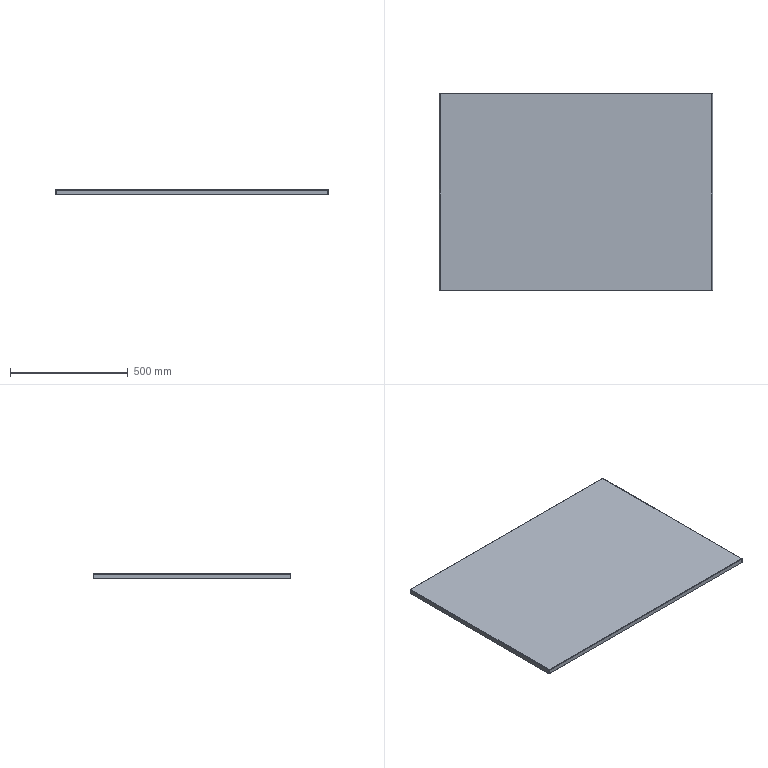Part | STEP file | Part 15 | 1 solid | 38 faces | box 1160 x 840 x 20 mm | volume 2086843 mm3 | plane 22 | spline 8 | cylinder 8 | commonest cylinder face diameters 1 x4 5 x4
STEP:
#1=CARTESIAN_POINT('',(-577.5,-417.5,-2.));
#2=VERTEX_POINT('',#1);
#3=CARTESIAN_POINT('',(577.5,-417.5,-2.));
#4=VERTEX_POINT('',#3);
#5=CARTESIAN_POINT('',(-577.5,-417.5,-2.));
#6=DIRECTION('',(1.,0.,0.));
#7=VECTOR('',#6,1000.);
#8=LINE('',#5,#7);
#9=EDGE_CURVE('',#2,#4,#8,.T.);
#10=ORIENTED_EDGE('',*,*,#9,.F.);
#11=CARTESIAN_POINT('',(-577.5,417.5,-2.));
#12=VERTEX_POINT('',#11);
#13=CARTESIAN_POINT('',(-577.5,417.5,-2.));
#14=DIRECTION('',(0.,-1.,0.));
#15=VECTOR('',#14,1000.);
#16=LINE('',#13,#15);
#17=EDGE_CURVE('',#12,#2,#16,.T.);
#18=ORIENTED_EDGE('',*,*,#17,.F.);
#19=CARTESIAN_POINT('',(577.5,417.5,-2.));
#20=VERTEX_POINT('',#19);
#21=CARTESIAN_POINT('',(577.5,417.5,-2.));
#22=DIRECTION('',(-1.,0.,0.));
#23=VECTOR('',#22,1000.);
#24=LINE('',#21,#23);
#25=EDGE_CURVE('',#20,#12,#24,.T.);
#26=ORIENTED_EDGE('',*,*,#25,.F.);
#27=CARTESIAN_POINT('',(577.5,-417.5,-2.));
#28=DIRECTION('',(0.,1.,0.));
#29=VECTOR('',#28,1000.);
#30=LINE('',#27,#29);
#31=EDGE_CURVE('',#4,#20,#30,.T.);
#32=ORIENTED_EDGE('',*,*,#31,.F.);
#33=EDGE_LOOP('',(#10,#18,#26,#32));
#34=FACE_OUTER_BOUND('',#33,.T.);
#35=CARTESIAN_POINT('',(0.,0.,-2.));
#36=DIRECTION('',(0.,0.,1.));
#37=DIRECTION('',(1.,0.,0.));
#38=AXIS2_PLACEMENT_3D('',#35,#36,#37);
#39=PLANE('',#38);
#40=ADVANCED_FACE('',(#34),#39,.F.);
#41=CARTESIAN_POINT('',(-577.5,417.5,0.));
#42=VERTEX_POINT('',#41);
#43=CARTESIAN_POINT('',(-577.5,-417.5,0.));
#44=VERTEX_POINT('',#43);
#45=CARTESIAN_POINT('',(-577.5,417.5,0.));
#46=DIRECTION('',(0.,-1.,0.));
#47=VECTOR('',#46,1000.);
#48=LINE('',#45,#47);
#49=EDGE_CURVE('',#42,#44,#48,.T.);
#50=ORIENTED_EDGE('',*,*,#49,.T.);
#51=CARTESIAN_POINT('',(577.5,-417.5,0.));
#52=VERTEX_POINT('',#51);
#53=CARTESIAN_POINT('',(-577.5,-417.5,0.));
#54=DIRECTION('',(1.,0.,0.));
#55=VECTOR('',#54,1000.);
#56=LINE('',#53,#55);
#57=EDGE_CURVE('',#44,#52,#56,.T.);
#58=ORIENTED_EDGE('',*,*,#57,.T.);
#59=CARTESIAN_POINT('',(577.5,417.5,0.));
#60=VERTEX_POINT('',#59);
#61=CARTESIAN_POINT('',(577.5,-417.5,0.));
#62=DIRECTION('',(0.,1.,0.));
#63=VECTOR('',#62,1000.);
#64=LINE('',#61,#63);
#65=EDGE_CURVE('',#52,#60,#64,.T.);
#66=ORIENTED_EDGE('',*,*,#65,.T.);
#67=CARTESIAN_POINT('',(577.5,417.5,0.));
#68=DIRECTION('',(-1.,0.,0.));
#69=VECTOR('',#68,1000.);
#70=LINE('',#67,#69);
#71=EDGE_CURVE('',#60,#42,#70,.T.);
#72=ORIENTED_EDGE('',*,*,#71,.T.);
#73=EDGE_LOOP('',(#50,#58,#66,#72));
#74=FACE_OUTER_BOUND('',#73,.T.);
#75=CARTESIAN_POINT('',(0.,0.,0.));
#76=DIRECTION('',(0.,0.,1.));
#77=DIRECTION('',(1.,0.,0.));
#78=AXIS2_PLACEMENT_3D('',#75,#76,#77);
#79=PLANE('',#78);
#80=ADVANCED_FACE('',(#74),#79,.T.);
#81=CARTESIAN_POINT('',(-577.293,420.,-2.5));
#82=VERTEX_POINT('',#81);
#83=CARTESIAN_POINT('',(-577.293,418.,-2.5));
#84=VERTEX_POINT('',#83);
#85=CARTESIAN_POINT('',(-577.293,418.,-2.5));
#86=DIRECTION('',(0.,-1.,0.));
#87=VECTOR('',#86,1000.);
#88=LINE('',#85,#87);
#89=EDGE_CURVE('',#82,#84,#88,.T.);
#90=ORIENTED_EDGE('',*,*,#89,.T.);
#91=CARTESIAN_POINT('',(-577.5,417.5,-2.));
#92=CARTESIAN_POINT('',(-577.465,417.631,-2.));
#93=CARTESIAN_POINT('',(-577.431,417.761,-2.054));
#94=CARTESIAN_POINT('',(-577.362,417.946,-2.239));
#95=CARTESIAN_POINT('',(-577.327,418.,-2.369));
#96=CARTESIAN_POINT('',(-577.293,418.,-2.5));
#97=B_SPLINE_CURVE_WITH_KNOTS('',3,(#91,#92,#93,#94,#95,#96),.UNSPECIFIED.,.F.,.F.,(4,2,4),(0.,0.5,1.),.UNSPECIFIED.);
#98=EDGE_CURVE('',#12,#84,#97,.T.);
#99=ORIENTED_EDGE('',*,*,#98,.F.);
#100=CARTESIAN_POINT('',(-577.5,417.5,-2.));
#101=DIRECTION('',(0.,0.,1.));
#102=VECTOR('',#101,1000.);
#103=LINE('',#100,#102);
#104=EDGE_CURVE('',#12,#42,#103,.T.);
#105=ORIENTED_EDGE('',*,*,#104,.T.);
#106=CARTESIAN_POINT('',(-577.5,417.5,0.));
#107=CARTESIAN_POINT('',(-577.483,417.827,0.));
#108=CARTESIAN_POINT('',(-577.465,418.154,-0.06507));
#109=CARTESIAN_POINT('',(-577.431,418.759,-0.3155));
#110=CARTESIAN_POINT('',(-577.414,419.036,-0.5008));
#111=CARTESIAN_POINT('',(-577.379,419.499,-0.9636));
#112=CARTESIAN_POINT('',(-577.362,419.684,-1.241));
#113=CARTESIAN_POINT('',(-577.327,419.935,-1.846));
#114=CARTESIAN_POINT('',(-577.31,420.,-2.173));
#115=CARTESIAN_POINT('',(-577.293,420.,-2.5));
#116=B_SPLINE_CURVE_WITH_KNOTS('',3,(#106,#107,#108,#109,#110,#111,#112,#113,#114,#115),.UNSPECIFIED.,.F.,.F.,(4,2,2,2,4),(0.,0.25,0.5,0.75,1.),.UNSPECIFIED.);
#117=EDGE_CURVE('',#42,#82,#116,.T.);
#118=ORIENTED_EDGE('',*,*,#117,.T.);
#119=EDGE_LOOP('',(#90,#99,#105,#118));
#120=FACE_OUTER_BOUND('',#119,.T.);
#121=CARTESIAN_POINT('',(-577.5,417.5,0.02));
#122=CARTESIAN_POINT('',(-577.483,417.83,0.02));
#123=CARTESIAN_POINT('',(-577.465,418.16,-0.04559));
#124=CARTESIAN_POINT('',(-577.431,418.769,-0.2981));
#125=CARTESIAN_POINT('',(-577.414,419.049,-0.4848));
#126=CARTESIAN_POINT('',(-577.379,419.515,-0.9513));
#127=CARTESIAN_POINT('',(-577.362,419.702,-1.231));
#128=CARTESIAN_POINT('',(-577.327,419.954,-1.84));
#129=CARTESIAN_POINT('',(-577.31,420.02,-2.17));
#130=CARTESIAN_POINT('',(-577.293,420.02,-2.5));
#131=CARTESIAN_POINT('',(-577.5,417.5,0.));
#132=CARTESIAN_POINT('',(-577.483,417.827,0.));
#133=CARTESIAN_POINT('',(-577.465,418.154,-0.06507));
#134=CARTESIAN_POINT('',(-577.431,418.759,-0.3155));
#135=CARTESIAN_POINT('',(-577.414,419.036,-0.5008));
#136=CARTESIAN_POINT('',(-577.379,419.499,-0.9636));
#137=CARTESIAN_POINT('',(-577.362,419.684,-1.241));
#138=CARTESIAN_POINT('',(-577.327,419.935,-1.846));
#139=CARTESIAN_POINT('',(-577.31,420.,-2.173));
#140=CARTESIAN_POINT('',(-577.293,420.,-2.5));
#141=CARTESIAN_POINT('',(-577.5,417.5,-2.));
#142=CARTESIAN_POINT('',(-577.483,417.565,-2.));
#143=CARTESIAN_POINT('',(-577.465,417.631,-2.013));
#144=CARTESIAN_POINT('',(-577.431,417.752,-2.063));
#145=CARTESIAN_POINT('',(-577.414,417.807,-2.1));
#146=CARTESIAN_POINT('',(-577.379,417.9,-2.193));
#147=CARTESIAN_POINT('',(-577.362,417.937,-2.248));
#148=CARTESIAN_POINT('',(-577.327,417.987,-2.369));
#149=CARTESIAN_POINT('',(-577.31,418.,-2.435));
#150=CARTESIAN_POINT('',(-577.293,418.,-2.5));
#151=CARTESIAN_POINT('',(-577.5,417.5,-2.02));
#152=CARTESIAN_POINT('',(-577.483,417.563,-2.02));
#153=CARTESIAN_POINT('',(-577.465,417.626,-2.033));
#154=CARTESIAN_POINT('',(-577.431,417.742,-2.081));
#155=CARTESIAN_POINT('',(-577.414,417.795,-2.116));
#156=CARTESIAN_POINT('',(-577.379,417.884,-2.205));
#157=CARTESIAN_POINT('',(-577.362,417.919,-2.258));
#158=CARTESIAN_POINT('',(-577.327,417.967,-2.374));
#159=CARTESIAN_POINT('',(-577.31,417.98,-2.437));
#160=CARTESIAN_POINT('',(-577.293,417.98,-2.5));
#161=B_SPLINE_SURFACE_WITH_KNOTS('',1,3,((#121,#122,#123,#124,#125,#126,#127,#128,#129,#130),(#131,#132,#133,#134,#135,#136,#137,#138,#139,#140),(#141,#142,#143,#144,#145,#146,#147,#148,#149,#150),(#151,#152,#153,#154,#155,#156,#157,#158,#159,#160)),.UNSPECIFIED.,.F.,.F.,.F.,(2,1,1,2),(4,2,2,2,4),(-0.01,0.,1.,1.01),(0.,0.25,0.5,0.75,1.),.UNSPECIFIED.);
#162=ADVANCED_FACE('',(#120),#161,.F.);
#163=CARTESIAN_POINT('',(577.293,418.,-2.5));
#164=VERTEX_POINT('',#163);
#165=CARTESIAN_POINT('',(577.293,418.,-2.5));
#166=CARTESIAN_POINT('',(577.327,418.,-2.369));
#167=CARTESIAN_POINT('',(577.362,417.946,-2.239));
#168=CARTESIAN_POINT('',(577.431,417.761,-2.054));
#169=CARTESIAN_POINT('',(577.465,417.631,-2.));
#170=CARTESIAN_POINT('',(577.5,417.5,-2.));
#171=B_SPLINE_CURVE_WITH_KNOTS('',3,(#165,#166,#167,#168,#169,#170),.UNSPECIFIED.,.F.,.F.,(4,2,4),(0.,0.5,1.),.UNSPECIFIED.);
#172=EDGE_CURVE('',#164,#20,#171,.T.);
#173=ORIENTED_EDGE('',*,*,#172,.F.);
#174=CARTESIAN_POINT('',(577.293,420.,-2.5));
#175=VERTEX_POINT('',#174);
#176=CARTESIAN_POINT('',(577.293,418.,-2.5));
#177=DIRECTION('',(0.,-1.,0.));
#178=VECTOR('',#177,1000.);
#179=LINE('',#176,#178);
#180=EDGE_CURVE('',#175,#164,#179,.T.);
#181=ORIENTED_EDGE('',*,*,#180,.F.);
#182=CARTESIAN_POINT('',(577.293,420.,-2.5));
#183=CARTESIAN_POINT('',(577.31,420.,-2.173));
#184=CARTESIAN_POINT('',(577.327,419.935,-1.846));
#185=CARTESIAN_POINT('',(577.362,419.684,-1.241));
#186=CARTESIAN_POINT('',(577.379,419.499,-0.9636));
#187=CARTESIAN_POINT('',(577.414,419.036,-0.5008));
#188=CARTESIAN_POINT('',(577.431,418.759,-0.3155));
#189=CARTESIAN_POINT('',(577.465,418.154,-0.06507));
#190=CARTESIAN_POINT('',(577.483,417.827,0.));
#191=CARTESIAN_POINT('',(577.5,417.5,0.));
#192=B_SPLINE_CURVE_WITH_KNOTS('',3,(#182,#183,#184,#185,#186,#187,#188,#189,#190,#191),.UNSPECIFIED.,.F.,.F.,(4,2,2,2,4),(0.,0.25,0.5,0.75,1.),.UNSPECIFIED.);
#193=EDGE_CURVE('',#175,#60,#192,.T.);
#194=ORIENTED_EDGE('',*,*,#193,.T.);
#195=CARTESIAN_POINT('',(577.5,417.5,-2.));
#196=DIRECTION('',(0.,0.,1.));
#197=VECTOR('',#196,1000.);
#198=LINE('',#195,#197);
#199=EDGE_CURVE('',#20,#60,#198,.T.);
#200=ORIENTED_EDGE('',*,*,#199,.F.);
#201=EDGE_LOOP('',(#173,#181,#194,#200));
#202=FACE_OUTER_BOUND('',#201,.T.);
#203=CARTESIAN_POINT('',(577.293,420.02,-2.5));
#204=CARTESIAN_POINT('',(577.31,420.02,-2.17));
#205=CARTESIAN_POINT('',(577.327,419.954,-1.84));
#206=CARTESIAN_POINT('',(577.362,419.702,-1.231));
#207=CARTESIAN_POINT('',(577.379,419.515,-0.9513));
#208=CARTESIAN_POINT('',(577.414,419.049,-0.4848));
#209=CARTESIAN_POINT('',(577.431,418.769,-0.2981));
#210=CARTESIAN_POINT('',(577.465,418.16,-0.04559));
#211=CARTESIAN_POINT('',(577.483,417.83,0.02));
#212=CARTESIAN_POINT('',(577.5,417.5,0.02));
#213=CARTESIAN_POINT('',(577.293,420.,-2.5));
#214=CARTESIAN_POINT('',(577.31,420.,-2.173));
#215=CARTESIAN_POINT('',(577.327,419.935,-1.846));
#216=CARTESIAN_POINT('',(577.362,419.684,-1.241));
#217=CARTESIAN_POINT('',(577.379,419.499,-0.9636));
#218=CARTESIAN_POINT('',(577.414,419.036,-0.5008));
#219=CARTESIAN_POINT('',(577.431,418.759,-0.3155));
#220=CARTESIAN_POINT('',(577.465,418.154,-0.06507));
#221=CARTESIAN_POINT('',(577.483,417.827,0.));
#222=CARTESIAN_POINT('',(577.5,417.5,0.));
#223=CARTESIAN_POINT('',(577.293,418.,-2.5));
#224=CARTESIAN_POINT('',(577.31,418.,-2.435));
#225=CARTESIAN_POINT('',(577.327,417.987,-2.369));
#226=CARTESIAN_POINT('',(577.362,417.937,-2.248));
#227=CARTESIAN_POINT('',(577.379,417.9,-2.193));
#228=CARTESIAN_POINT('',(577.414,417.807,-2.1));
#229=CARTESIAN_POINT('',(577.431,417.752,-2.063));
#230=CARTESIAN_POINT('',(577.465,417.631,-2.013));
#231=CARTESIAN_POINT('',(577.483,417.565,-2.));
#232=CARTESIAN_POINT('',(577.5,417.5,-2.));
#233=CARTESIAN_POINT('',(577.293,417.98,-2.5));
#234=CARTESIAN_POINT('',(577.31,417.98,-2.437));
#235=CARTESIAN_POINT('',(577.327,417.967,-2.374));
#236=CARTESIAN_POINT('',(577.362,417.919,-2.258));
#237=CARTESIAN_POINT('',(577.379,417.884,-2.205));
#238=CARTESIAN_POINT('',(577.414,417.795,-2.116));
#239=CARTESIAN_POINT('',(577.431,417.742,-2.081));
#240=CARTESIAN_POINT('',(577.465,417.626,-2.033));
#241=CARTESIAN_POINT('',(577.483,417.563,-2.02));
#242=CARTESIAN_POINT('',(577.5,417.5,-2.02));
#243=B_SPLINE_SURFACE_WITH_KNOTS('',1,3,((#203,#204,#205,#206,#207,#208,#209,#210,#211,#212),(#213,#214,#215,#216,#217,#218,#219,#220,#221,#222),(#223,#224,#225,#226,#227,#228,#229,#230,#231,#232),(#233,#234,#235,#236,#237,#238,#239,#240,#241,#242)),.UNSPECIFIED.,.F.,.F.,.F.,(2,1,1,2),(4,2,2,2,4),(-0.01,0.,1.,1.01),(0.,0.25,0.5,0.75,1.),.UNSPECIFIED.);
#244=ADVANCED_FACE('',(#202),#243,.F.);
#245=ORIENTED_EDGE('',*,*,#71,.F.);
#246=ORIENTED_EDGE('',*,*,#193,.F.);
#247=CARTESIAN_POINT('',(0.,420.,-2.5));
#248=DIRECTION('',(1.,0.,0.));
#249=VECTOR('',#248,1000.);
#250=LINE('',#247,#249);
#251=EDGE_CURVE('',#82,#175,#250,.T.);
#252=ORIENTED_EDGE('',*,*,#251,.F.);
#253=ORIENTED_EDGE('',*,*,#117,.F.);
#254=EDGE_LOOP('',(#245,#246,#252,#253));
#255=FACE_OUTER_BOUND('',#254,.T.);
#256=CARTESIAN_POINT('',(577.5,417.5,-2.5));
#257=DIRECTION('',(1.,0.,0.));
#258=DIRECTION('',(0.,1.,0.));
#259=AXIS2_PLACEMENT_3D('',#256,#257,#258);
#260=CYLINDRICAL_SURFACE('',#259,2.5);
#261=ADVANCED_FACE('',(#255),#260,.T.);
#262=ORIENTED_EDGE('',*,*,#25,.T.);
#263=ORIENTED_EDGE('',*,*,#98,.T.);
#264=CARTESIAN_POINT('',(-580.,418.,-2.5));
#265=DIRECTION('',(1.,0.,0.));
#266=VECTOR('',#265,1000.);
#267=LINE('',#264,#266);
#268=EDGE_CURVE('',#84,#164,#267,.T.);
#269=ORIENTED_EDGE('',*,*,#268,.T.);
#270=ORIENTED_EDGE('',*,*,#172,.T.);
#271=EDGE_LOOP('',(#262,#263,#269,#270));
#272=FACE_OUTER_BOUND('',#271,.T.);
#273=CARTESIAN_POINT('',(577.5,417.5,-2.5));
#274=DIRECTION('',(1.,0.,0.));
#275=DIRECTION('',(0.,1.,0.));
#276=AXIS2_PLACEMENT_3D('',#273,#274,#275);
#277=CYLINDRICAL_SURFACE('',#276,0.5);
#278=ADVANCED_FACE('',(#272),#277,.F.);
#279=CARTESIAN_POINT('',(-577.293,418.,-20.));
#280=VERTEX_POINT('',#279);
#281=CARTESIAN_POINT('',(-577.293,420.,-20.));
#282=VERTEX_POINT('',#281);
#283=CARTESIAN_POINT('',(-577.293,420.,-20.));
#284=DIRECTION('',(0.,1.,0.));
#285=VECTOR('',#284,1000.);
#286=LINE('',#283,#285);
#287=EDGE_CURVE('',#280,#282,#286,.T.);
#288=ORIENTED_EDGE('',*,*,#287,.F.);
#289=CARTESIAN_POINT('',(-577.293,418.,0.));
#290=DIRECTION('',(0.,0.,-1.));
#291=VECTOR('',#290,1000.);
#292=LINE('',#289,#291);
#293=EDGE_CURVE('',#84,#280,#292,.T.);
#294=ORIENTED_EDGE('',*,*,#293,.F.);
#295=ORIENTED_EDGE('',*,*,#89,.F.);
#296=CARTESIAN_POINT('',(-577.293,420.,0.));
#297=DIRECTION('',(0.,0.,1.));
#298=VECTOR('',#297,1000.);
#299=LINE('',#296,#298);
#300=EDGE_CURVE('',#282,#82,#299,.T.);
#301=ORIENTED_EDGE('',*,*,#300,.F.);
#302=EDGE_LOOP('',(#288,#294,#295,#301));
#303=FACE_OUTER_BOUND('',#302,.T.);
#304=CARTESIAN_POINT('',(-577.293,418.,-2.));
#305=DIRECTION('',(-1.,0.,0.));
#306=DIRECTION('',(0.,0.,1.));
#307=AXIS2_PLACEMENT_3D('',#304,#305,#306);
#308=PLANE('',#307);
#309=ADVANCED_FACE('',(#303),#308,.T.);
#310=CARTESIAN_POINT('',(577.293,420.,-20.));
#311=VERTEX_POINT('',#310);
#312=CARTESIAN_POINT('',(577.293,420.,-2.));
#313=DIRECTION('',(0.,0.,1.));
#314=VECTOR('',#313,1000.);
#315=LINE('',#312,#314);
#316=EDGE_CURVE('',#311,#175,#315,.T.);
#317=ORIENTED_EDGE('',*,*,#316,.F.);
#318=CARTESIAN_POINT('',(580.,420.,-20.));
#319=DIRECTION('',(1.,0.,0.));
#320=VECTOR('',#319,1000.);
#321=LINE('',#318,#320);
#322=EDGE_CURVE('',#282,#311,#321,.T.);
#323=ORIENTED_EDGE('',*,*,#322,.F.);
#324=ORIENTED_EDGE('',*,*,#300,.T.);
#325=ORIENTED_EDGE('',*,*,#251,.T.);
#326=EDGE_LOOP('',(#317,#323,#324,#325));
#327=FACE_OUTER_BOUND('',#326,.T.);
#328=CARTESIAN_POINT('',(0.,420.,0.));
#329=DIRECTION('',(0.,1.,0.));
#330=DIRECTION('',(0.,0.,1.));
#331=AXIS2_PLACEMENT_3D('',#328,#329,#330);
#332=PLANE('',#331);
#333=ADVANCED_FACE('',(#327),#332,.T.);
#334=CARTESIAN_POINT('',(577.293,418.,-20.));
#335=VERTEX_POINT('',#334);
#336=CARTESIAN_POINT('',(0.,418.,-20.));
#337=DIRECTION('',(1.,0.,0.));
#338=VECTOR('',#337,1000.);
#339=LINE('',#336,#338);
#340=EDGE_CURVE('',#280,#335,#339,.T.);
#341=ORIENTED_EDGE('',*,*,#340,.T.);
#342=CARTESIAN_POINT('',(577.293,418.,-2.));
#343=DIRECTION('',(0.,0.,-1.));
#344=VECTOR('',#343,1000.);
#345=LINE('',#342,#344);
#346=EDGE_CURVE('',#164,#335,#345,.T.);
#347=ORIENTED_EDGE('',*,*,#346,.F.);
#348=ORIENTED_EDGE('',*,*,#268,.F.);
#349=ORIENTED_EDGE('',*,*,#293,.T.);
#350=EDGE_LOOP('',(#341,#347,#348,#349));
#351=FACE_OUTER_BOUND('',#350,.T.);
#352=CARTESIAN_POINT('',(0.,418.,0.));
#353=DIRECTION('',(0.,1.,0.));
#354=DIRECTION('',(0.,0.,1.));
#355=AXIS2_PLACEMENT_3D('',#352,#353,#354);
#356=PLANE('',#355);
#357=ADVANCED_FACE('',(#351),#356,.F.);
#358=CARTESIAN_POINT('',(577.293,418.,-20.));
#359=DIRECTION('',(0.,1.,0.));
#360=VECTOR('',#359,1000.);
#361=LINE('',#358,#360);
#362=EDGE_CURVE('',#335,#311,#361,.T.);
#363=ORIENTED_EDGE('',*,*,#362,.F.);
#364=ORIENTED_EDGE('',*,*,#340,.F.);
#365=ORIENTED_EDGE('',*,*,#287,.T.);
#366=ORIENTED_EDGE('',*,*,#322,.T.);
#367=EDGE_LOOP('',(#363,#364,#365,#366));
#368=FACE_OUTER_BOUND('',#367,.T.);
#369=CARTESIAN_POINT('',(580.,420.,-20.));
#370=DIRECTION('',(0.,0.,-1.));
#371=DIRECTION('',(0.,1.,0.));
#372=AXIS2_PLACEMENT_3D('',#369,#370,#371);
#373=PLANE('',#372);
#374=ADVANCED_FACE('',(#368),#373,.T.);
#375=ORIENTED_EDGE('',*,*,#346,.T.);
#376=ORIENTED_EDGE('',*,*,#362,.T.);
#377=ORIENTED_EDGE('',*,*,#316,.T.);
#378=ORIENTED_EDGE('',*,*,#180,.T.);
#379=EDGE_LOOP('',(#375,#376,#377,#378));
#380=FACE_OUTER_BOUND('',#379,.T.);
#381=CARTESIAN_POINT('',(577.293,418.,-2.));
#382=DIRECTION('',(-1.,0.,0.));
#383=DIRECTION('',(0.,0.,1.));
#384=AXIS2_PLACEMENT_3D('',#381,#382,#383);
#385=PLANE('',#384);
#386=ADVANCED_FACE('',(#380),#385,.F.);
#387=CARTESIAN_POINT('',(580.,417.293,-2.5));
#388=VERTEX_POINT('',#387);
#389=CARTESIAN_POINT('',(578.,417.293,-2.5));
#390=VERTEX_POINT('',#389);
#391=CARTESIAN_POINT('',(578.,417.293,-2.5));
#392=DIRECTION('',(-1.,0.,0.));
#393=VECTOR('',#392,1000.);
#394=LINE('',#391,#393);
#395=EDGE_CURVE('',#388,#390,#394,.T.);
#396=ORIENTED_EDGE('',*,*,#395,.T.);
#397=CARTESIAN_POINT('',(577.5,417.5,-2.));
#398=CARTESIAN_POINT('',(577.631,417.465,-2.));
#399=CARTESIAN_POINT('',(577.761,417.431,-2.054));
#400=CARTESIAN_POINT('',(577.946,417.362,-2.239));
#401=CARTESIAN_POINT('',(578.,417.327,-2.369));
#402=CARTESIAN_POINT('',(578.,417.293,-2.5));
#403=B_SPLINE_CURVE_WITH_KNOTS('',3,(#397,#398,#399,#400,#401,#402),.UNSPECIFIED.,.F.,.F.,(4,2,4),(0.,0.5,1.),.UNSPECIFIED.);
#404=EDGE_CURVE('',#20,#390,#403,.T.);
#405=ORIENTED_EDGE('',*,*,#404,.F.);
#406=ORIENTED_EDGE('',*,*,#199,.T.);
#407=CARTESIAN_POINT('',(577.5,417.5,0.));
#408=CARTESIAN_POINT('',(577.827,417.483,0.));
#409=CARTESIAN_POINT('',(578.154,417.465,-0.06507));
#410=CARTESIAN_POINT('',(578.759,417.431,-0.3155));
#411=CARTESIAN_POINT('',(579.036,417.414,-0.5008));
#412=CARTESIAN_POINT('',(579.499,417.379,-0.9636));
#413=CARTESIAN_POINT('',(579.684,417.362,-1.241));
#414=CARTESIAN_POINT('',(579.935,417.327,-1.846));
#415=CARTESIAN_POINT('',(580.,417.31,-2.173));
#416=CARTESIAN_POINT('',(580.,417.293,-2.5));
#417=B_SPLINE_CURVE_WITH_KNOTS('',3,(#407,#408,#409,#410,#411,#412,#413,#414,#415,#416),.UNSPECIFIED.,.F.,.F.,(4,2,2,2,4),(0.,0.25,0.5,0.75,1.),.UNSPECIFIED.);
#418=EDGE_CURVE('',#60,#388,#417,.T.);
#419=ORIENTED_EDGE('',*,*,#418,.T.);
#420=EDGE_LOOP('',(#396,#405,#406,#419));
#421=FACE_OUTER_BOUND('',#420,.T.);
#422=CARTESIAN_POINT('',(577.5,417.5,0.02));
#423=CARTESIAN_POINT('',(577.83,417.483,0.02));
#424=CARTESIAN_POINT('',(578.16,417.465,-0.04559));
#425=CARTESIAN_POINT('',(578.769,417.431,-0.2981));
#426=CARTESIAN_POINT('',(579.049,417.414,-0.4848));
#427=CARTESIAN_POINT('',(579.515,417.379,-0.9513));
#428=CARTESIAN_POINT('',(579.702,417.362,-1.231));
#429=CARTESIAN_POINT('',(579.954,417.327,-1.84));
#430=CARTESIAN_POINT('',(580.02,417.31,-2.17));
#431=CARTESIAN_POINT('',(580.02,417.293,-2.5));
#432=CARTESIAN_POINT('',(577.5,417.5,0.));
#433=CARTESIAN_POINT('',(577.827,417.483,0.));
#434=CARTESIAN_POINT('',(578.154,417.465,-0.06507));
#435=CARTESIAN_POINT('',(578.759,417.431,-0.3155));
#436=CARTESIAN_POINT('',(579.036,417.414,-0.5008));
#437=CARTESIAN_POINT('',(579.499,417.379,-0.9636));
#438=CARTESIAN_POINT('',(579.684,417.362,-1.241));
#439=CARTESIAN_POINT('',(579.935,417.327,-1.846));
#440=CARTESIAN_POINT('',(580.,417.31,-2.173));
#441=CARTESIAN_POINT('',(580.,417.293,-2.5));
#442=CARTESIAN_POINT('',(577.5,417.5,-2.));
#443=CARTESIAN_POINT('',(577.565,417.483,-2.));
#444=CARTESIAN_POINT('',(577.631,417.465,-2.013));
#445=CARTESIAN_POINT('',(577.752,417.431,-2.063));
#446=CARTESIAN_POINT('',(577.807,417.414,-2.1));
#447=CARTESIAN_POINT('',(577.9,417.379,-2.193));
#448=CARTESIAN_POINT('',(577.937,417.362,-2.248));
#449=CARTESIAN_POINT('',(577.987,417.327,-2.369));
#450=CARTESIAN_POINT('',(578.,417.31,-2.435));
#451=CARTESIAN_POINT('',(578.,417.293,-2.5));
#452=CARTESIAN_POINT('',(577.5,417.5,-2.02));
#453=CARTESIAN_POINT('',(577.563,417.483,-2.02));
#454=CARTESIAN_POINT('',(577.626,417.465,-2.033));
#455=CARTESIAN_POINT('',(577.742,417.431,-2.081));
#456=CARTESIAN_POINT('',(577.795,417.414,-2.116));
#457=CARTESIAN_POINT('',(577.884,417.379,-2.205));
#458=CARTESIAN_POINT('',(577.919,417.362,-2.258));
#459=CARTESIAN_POINT('',(577.967,417.327,-2.374));
#460=CARTESIAN_POINT('',(577.98,417.31,-2.437));
#461=CARTESIAN_POINT('',(577.98,417.293,-2.5));
#462=B_SPLINE_SURFACE_WITH_KNOTS('',1,3,((#422,#423,#424,#425,#426,#427,#428,#429,#430,#431),(#432,#433,#434,#435,#436,#437,#438,#439,#440,#441),(#442,#443,#444,#445,#446,#447,#448,#449,#450,#451),(#452,#453,#454,#455,#456,#457,#458,#459,#460,#461)),.UNSPECIFIED.,.F.,.F.,.F.,(2,1,1,2),(4,2,2,2,4),(-0.01,0.,1.,1.01),(0.,0.25,0.5,0.75,1.),.UNSPECIFIED.);
#463=ADVANCED_FACE('',(#421),#462,.F.);
#464=CARTESIAN_POINT('',(578.,-417.293,-2.5));
#465=VERTEX_POINT('',#464);
#466=CARTESIAN_POINT('',(578.,-417.293,-2.5));
#467=CARTESIAN_POINT('',(578.,-417.327,-2.369));
#468=CARTESIAN_POINT('',(577.946,-417.362,-2.239));
#469=CARTESIAN_POINT('',(577.761,-417.431,-2.054));
#470=CARTESIAN_POINT('',(577.631,-417.465,-2.));
#471=CARTESIAN_POINT('',(577.5,-417.5,-2.));
#472=B_SPLINE_CURVE_WITH_KNOTS('',3,(#466,#467,#468,#469,#470,#471),.UNSPECIFIED.,.F.,.F.,(4,2,4),(0.,0.5,1.),.UNSPECIFIED.);
#473=EDGE_CURVE('',#465,#4,#472,.T.);
#474=ORIENTED_EDGE('',*,*,#473,.F.);
#475=CARTESIAN_POINT('',(580.,-417.293,-2.5));
#476=VERTEX_POINT('',#475);
#477=CARTESIAN_POINT('',(578.,-417.293,-2.5));
#478=DIRECTION('',(-1.,0.,0.));
#479=VECTOR('',#478,1000.);
#480=LINE('',#477,#479);
#481=EDGE_CURVE('',#476,#465,#480,.T.);
#482=ORIENTED_EDGE('',*,*,#481,.F.);
#483=CARTESIAN_POINT('',(580.,-417.293,-2.5));
#484=CARTESIAN_POINT('',(580.,-417.31,-2.173));
#485=CARTESIAN_POINT('',(579.935,-417.327,-1.846));
#486=CARTESIAN_POINT('',(579.684,-417.362,-1.241));
#487=CARTESIAN_POINT('',(579.499,-417.379,-0.9636));
#488=CARTESIAN_POINT('',(579.036,-417.414,-0.5008));
#489=CARTESIAN_POINT('',(578.759,-417.431,-0.3155));
#490=CARTESIAN_POINT('',(578.154,-417.465,-0.06507));
#491=CARTESIAN_POINT('',(577.827,-417.483,0.));
#492=CARTESIAN_POINT('',(577.5,-417.5,0.));
#493=B_SPLINE_CURVE_WITH_KNOTS('',3,(#483,#484,#485,#486,#487,#488,#489,#490,#491,#492),.UNSPECIFIED.,.F.,.F.,(4,2,2,2,4),(0.,0.25,0.5,0.75,1.),.UNSPECIFIED.);
#494=EDGE_CURVE('',#476,#52,#493,.T.);
#495=ORIENTED_EDGE('',*,*,#494,.T.);
#496=CARTESIAN_POINT('',(577.5,-417.5,-2.));
#497=DIRECTION('',(0.,0.,1.));
#498=VECTOR('',#497,1000.);
#499=LINE('',#496,#498);
#500=EDGE_CURVE('',#4,#52,#499,.T.);
#501=ORIENTED_EDGE('',*,*,#500,.F.);
#502=EDGE_LOOP('',(#474,#482,#495,#501));
#503=FACE_OUTER_BOUND('',#502,.T.);
#504=CARTESIAN_POINT('',(580.02,-417.293,-2.5));
#505=CARTESIAN_POINT('',(580.02,-417.31,-2.17));
#506=CARTESIAN_POINT('',(579.954,-417.327,-1.84));
#507=CARTESIAN_POINT('',(579.702,-417.362,-1.231));
#508=CARTESIAN_POINT('',(579.515,-417.379,-0.9513));
#509=CARTESIAN_POINT('',(579.049,-417.414,-0.4848));
#510=CARTESIAN_POINT('',(578.769,-417.431,-0.2981));
#511=CARTESIAN_POINT('',(578.16,-417.465,-0.04559));
#512=CARTESIAN_POINT('',(577.83,-417.483,0.02));
#513=CARTESIAN_POINT('',(577.5,-417.5,0.02));
#514=CARTESIAN_POINT('',(580.,-417.293,-2.5));
#515=CARTESIAN_POINT('',(580.,-417.31,-2.173));
#516=CARTESIAN_POINT('',(579.935,-417.327,-1.846));
#517=CARTESIAN_POINT('',(579.684,-417.362,-1.241));
#518=CARTESIAN_POINT('',(579.499,-417.379,-0.9636));
#519=CARTESIAN_POINT('',(579.036,-417.414,-0.5008));
#520=CARTESIAN_POINT('',(578.759,-417.431,-0.3155));
#521=CARTESIAN_POINT('',(578.154,-417.465,-0.06507));
#522=CARTESIAN_POINT('',(577.827,-417.483,0.));
#523=CARTESIAN_POINT('',(577.5,-417.5,0.));
#524=CARTESIAN_POINT('',(578.,-417.293,-2.5));
#525=CARTESIAN_POINT('',(578.,-417.31,-2.435));
#526=CARTESIAN_POINT('',(577.987,-417.327,-2.369));
#527=CARTESIAN_POINT('',(577.937,-417.362,-2.248));
#528=CARTESIAN_POINT('',(577.9,-417.379,-2.193));
#529=CARTESIAN_POINT('',(577.807,-417.414,-2.1));
#530=CARTESIAN_POINT('',(577.752,-417.431,-2.063));
#531=CARTESIAN_POINT('',(577.631,-417.465,-2.013));
#532=CARTESIAN_POINT('',(577.565,-417.483,-2.));
#533=CARTESIAN_POINT('',(577.5,-417.5,-2.));
#534=CARTESIAN_POINT('',(577.98,-417.293,-2.5));
#535=CARTESIAN_POINT('',(577.98,-417.31,-2.437));
#536=CARTESIAN_POINT('',(577.967,-417.327,-2.374));
#537=CARTESIAN_POINT('',(577.919,-417.362,-2.258));
#538=CARTESIAN_POINT('',(577.884,-417.379,-2.205));
#539=CARTESIAN_POINT('',(577.795,-417.414,-2.116));
#540=CARTESIAN_POINT('',(577.742,-417.431,-2.081));
#541=CARTESIAN_POINT('',(577.626,-417.465,-2.033));
#542=CARTESIAN_POINT('',(577.563,-417.483,-2.02));
#543=CARTESIAN_POINT('',(577.5,-417.5,-2.02));
#544=B_SPLINE_SURFACE_WITH_KNOTS('',1,3,((#504,#505,#506,#507,#508,#509,#510,#511,#512,#513),(#514,#515,#516,#517,#518,#519,#520,#521,#522,#523),(#524,#525,#526,#527,#528,#529,#530,#531,#532,#533),(#534,#535,#536,#537,#538,#539,#540,#541,#542,#543)),.UNSPECIFIED.,.F.,.F.,.F.,(2,1,1,2),(4,2,2,2,4),(-0.01,0.,1.,1.01),(0.,0.25,0.5,0.75,1.),.UNSPECIFIED.);
#545=ADVANCED_FACE('',(#503),#544,.F.);
#546=ORIENTED_EDGE('',*,*,#65,.F.);
#547=ORIENTED_EDGE('',*,*,#494,.F.);
#548=CARTESIAN_POINT('',(580.,420.,-2.5));
#549=DIRECTION('',(0.,1.,0.));
#550=VECTOR('',#549,1000.);
#551=LINE('',#548,#550);
#552=EDGE_CURVE('',#476,#388,#551,.T.);
#553=ORIENTED_EDGE('',*,*,#552,.T.);
#554=ORIENTED_EDGE('',*,*,#418,.F.);
#555=EDGE_LOOP('',(#546,#547,#553,#554));
#556=FACE_OUTER_BOUND('',#555,.T.);
#557=CARTESIAN_POINT('',(577.5,-417.5,-2.5));
#558=DIRECTION('',(0.,-1.,0.));
#559=DIRECTION('',(1.,0.,0.));
#560=AXIS2_PLACEMENT_3D('',#557,#558,#559);
#561=CYLINDRICAL_SURFACE('',#560,2.5);
#562=ADVANCED_FACE('',(#556),#561,.T.);
#563=ORIENTED_EDGE('',*,*,#31,.T.);
#564=ORIENTED_EDGE('',*,*,#404,.T.);
#565=CARTESIAN_POINT('',(578.,420.,-2.5));
#566=DIRECTION('',(0.,-1.,0.));
#567=VECTOR('',#566,1000.);
#568=LINE('',#565,#567);
#569=EDGE_CURVE('',#390,#465,#568,.T.);
#570=ORIENTED_EDGE('',*,*,#569,.T.);
#571=ORIENTED_EDGE('',*,*,#473,.T.);
#572=EDGE_LOOP('',(#563,#564,#570,#571));
#573=FACE_OUTER_BOUND('',#572,.T.);
#574=CARTESIAN_POINT('',(577.5,-417.5,-2.5));
#575=DIRECTION('',(0.,-1.,0.));
#576=DIRECTION('',(1.,0.,0.));
#577=AXIS2_PLACEMENT_3D('',#574,#575,#576);
#578=CYLINDRICAL_SURFACE('',#577,0.5);
#579=ADVANCED_FACE('',(#573),#578,.F.);
#580=CARTESIAN_POINT('',(578.,417.293,-20.));
#581=VERTEX_POINT('',#580);
#582=CARTESIAN_POINT('',(580.,417.293,-20.));
#583=VERTEX_POINT('',#582);
#584=CARTESIAN_POINT('',(580.,417.293,-20.));
#585=DIRECTION('',(1.,0.,0.));
#586=VECTOR('',#585,1000.);
#587=LINE('',#584,#586);
#588=EDGE_CURVE('',#581,#583,#587,.T.);
#589=ORIENTED_EDGE('',*,*,#588,.F.);
#590=CARTESIAN_POINT('',(578.,417.293,0.));
#591=DIRECTION('',(0.,0.,-1.));
#592=VECTOR('',#591,1000.);
#593=LINE('',#590,#592);
#594=EDGE_CURVE('',#390,#581,#593,.T.);
#595=ORIENTED_EDGE('',*,*,#594,.F.);
#596=ORIENTED_EDGE('',*,*,#395,.F.);
#597=CARTESIAN_POINT('',(580.,417.293,-2.));
#598=DIRECTION('',(0.,0.,-1.));
#599=VECTOR('',#598,1000.);
#600=LINE('',#597,#599);
#601=EDGE_CURVE('',#388,#583,#600,.T.);
#602=ORIENTED_EDGE('',*,*,#601,.T.);
#603=EDGE_LOOP('',(#589,#595,#596,#602));
#604=FACE_OUTER_BOUND('',#603,.T.);
#605=CARTESIAN_POINT('',(578.,417.293,-2.));
#606=DIRECTION('',(0.,1.,0.));
#607=DIRECTION('',(0.,0.,1.));
#608=AXIS2_PLACEMENT_3D('',#605,#606,#607);
#609=PLANE('',#608);
#610=ADVANCED_FACE('',(#604),#609,.T.);
#611=ORIENTED_EDGE('',*,*,#552,.F.);
#612=CARTESIAN_POINT('',(580.,-417.293,-20.));
#613=VERTEX_POINT('',#612);
#614=CARTESIAN_POINT('',(580.,-417.293,0.));
#615=DIRECTION('',(0.,0.,-1.));
#616=VECTOR('',#615,1000.);
#617=LINE('',#614,#616);
#618=EDGE_CURVE('',#476,#613,#617,.T.);
#619=ORIENTED_EDGE('',*,*,#618,.T.);
#620=CARTESIAN_POINT('',(580.,420.,-20.));
#621=DIRECTION('',(0.,-1.,0.));
#622=VECTOR('',#621,1000.);
#623=LINE('',#620,#622);
#624=EDGE_CURVE('',#583,#613,#623,.T.);
#625=ORIENTED_EDGE('',*,*,#624,.F.);
#626=ORIENTED_EDGE('',*,*,#601,.F.);
#627=EDGE_LOOP('',(#611,#619,#625,#626));
#628=FACE_OUTER_BOUND('',#627,.T.);
#629=CARTESIAN_POINT('',(580.,0.,0.));
#630=DIRECTION('',(-1.,0.,0.));
#631=DIRECTION('',(0.,0.,1.));
#632=AXIS2_PLACEMENT_3D('',#629,#630,#631);
#633=PLANE('',#632);
#634=ADVANCED_FACE('',(#628),#633,.F.);
#635=CARTESIAN_POINT('',(578.,-417.293,-20.));
#636=VERTEX_POINT('',#635);
#637=CARTESIAN_POINT('',(578.,-417.293,-2.));
#638=DIRECTION('',(0.,0.,-1.));
#639=VECTOR('',#638,1000.);
#640=LINE('',#637,#639);
#641=EDGE_CURVE('',#465,#636,#640,.T.);
#642=ORIENTED_EDGE('',*,*,#641,.F.);
#643=ORIENTED_EDGE('',*,*,#569,.F.);
#644=ORIENTED_EDGE('',*,*,#594,.T.);
#645=CARTESIAN_POINT('',(578.,0.,-20.));
#646=DIRECTION('',(0.,-1.,0.));
#647=VECTOR('',#646,1000.);
#648=LINE('',#645,#647);
#649=EDGE_CURVE('',#581,#636,#648,.T.);
#650=ORIENTED_EDGE('',*,*,#649,.T.);
#651=EDGE_LOOP('',(#642,#643,#644,#650));
#652=FACE_OUTER_BOUND('',#651,.T.);
#653=CARTESIAN_POINT('',(578.,0.,0.));
#654=DIRECTION('',(-1.,0.,0.));
#655=DIRECTION('',(0.,0.,1.));
#656=AXIS2_PLACEMENT_3D('',#653,#654,#655);
#657=PLANE('',#656);
#658=ADVANCED_FACE('',(#652),#657,.T.);
#659=CARTESIAN_POINT('',(578.,-417.293,-20.));
#660=DIRECTION('',(1.,0.,0.));
#661=VECTOR('',#660,1000.);
#662=LINE('',#659,#661);
#663=EDGE_CURVE('',#636,#613,#662,.T.);
#664=ORIENTED_EDGE('',*,*,#663,.F.);
#665=ORIENTED_EDGE('',*,*,#649,.F.);
#666=ORIENTED_EDGE('',*,*,#588,.T.);
#667=ORIENTED_EDGE('',*,*,#624,.T.);
#668=EDGE_LOOP('',(#664,#665,#666,#667));
#669=FACE_OUTER_BOUND('',#668,.T.);
#670=CARTESIAN_POINT('',(580.,420.,-20.));
#671=DIRECTION('',(0.,0.,-1.));
#672=DIRECTION('',(-1.,0.,0.));
#673=AXIS2_PLACEMENT_3D('',#670,#671,#672);
#674=PLANE('',#673);
#675=ADVANCED_FACE('',(#669),#674,.T.);
#676=ORIENTED_EDGE('',*,*,#641,.T.);
#677=ORIENTED_EDGE('',*,*,#663,.T.);
#678=ORIENTED_EDGE('',*,*,#618,.F.);
#679=ORIENTED_EDGE('',*,*,#481,.T.);
#680=EDGE_LOOP('',(#676,#677,#678,#679));
#681=FACE_OUTER_BOUND('',#680,.T.);
#682=CARTESIAN_POINT('',(578.,-417.293,-2.));
#683=DIRECTION('',(0.,1.,0.));
#684=DIRECTION('',(0.,0.,1.));
#685=AXIS2_PLACEMENT_3D('',#682,#683,#684);
#686=PLANE('',#685);
#687=ADVANCED_FACE('',(#681),#686,.F.);
#688=CARTESIAN_POINT('',(-580.,-417.293,-2.5));
#689=VERTEX_POINT('',#688);
#690=CARTESIAN_POINT('',(-578.,-417.293,-2.5));
#691=VERTEX_POINT('',#690);
#692=CARTESIAN_POINT('',(-578.,-417.293,-2.5));
#693=DIRECTION('',(1.,0.,0.));
#694=VECTOR('',#693,1000.);
#695=LINE('',#692,#694);
#696=EDGE_CURVE('',#689,#691,#695,.T.);
#697=ORIENTED_EDGE('',*,*,#696,.T.);
#698=CARTESIAN_POINT('',(-577.5,-417.5,-2.));
#699=CARTESIAN_POINT('',(-577.631,-417.465,-2.));
#700=CARTESIAN_POINT('',(-577.761,-417.431,-2.054));
#701=CARTESIAN_POINT('',(-577.946,-417.362,-2.239));
#702=CARTESIAN_POINT('',(-578.,-417.327,-2.369));
#703=CARTESIAN_POINT('',(-578.,-417.293,-2.5));
#704=B_SPLINE_CURVE_WITH_KNOTS('',3,(#698,#699,#700,#701,#702,#703),.UNSPECIFIED.,.F.,.F.,(4,2,4),(0.,0.5,1.),.UNSPECIFIED.);
#705=EDGE_CURVE('',#2,#691,#704,.T.);
#706=ORIENTED_EDGE('',*,*,#705,.F.);
#707=CARTESIAN_POINT('',(-577.5,-417.5,-2.));
#708=DIRECTION('',(0.,0.,1.));
#709=VECTOR('',#708,1000.);
#710=LINE('',#707,#709);
#711=EDGE_CURVE('',#2,#44,#710,.T.);
#712=ORIENTED_EDGE('',*,*,#711,.T.);
#713=CARTESIAN_POINT('',(-577.5,-417.5,0.));
#714=CARTESIAN_POINT('',(-577.827,-417.483,0.));
#715=CARTESIAN_POINT('',(-578.154,-417.465,-0.06507));
#716=CARTESIAN_POINT('',(-578.759,-417.431,-0.3155));
#717=CARTESIAN_POINT('',(-579.036,-417.414,-0.5008));
#718=CARTESIAN_POINT('',(-579.499,-417.379,-0.9636));
#719=CARTESIAN_POINT('',(-579.684,-417.362,-1.241));
#720=CARTESIAN_POINT('',(-579.935,-417.327,-1.846));
#721=CARTESIAN_POINT('',(-580.,-417.31,-2.173));
#722=CARTESIAN_POINT('',(-580.,-417.293,-2.5));
#723=B_SPLINE_CURVE_WITH_KNOTS('',3,(#713,#714,#715,#716,#717,#718,#719,#720,#721,#722),.UNSPECIFIED.,.F.,.F.,(4,2,2,2,4),(0.,0.25,0.5,0.75,1.),.UNSPECIFIED.);
#724=EDGE_CURVE('',#44,#689,#723,.T.);
#725=ORIENTED_EDGE('',*,*,#724,.T.);
#726=EDGE_LOOP('',(#697,#706,#712,#725));
#727=FACE_OUTER_BOUND('',#726,.T.);
#728=CARTESIAN_POINT('',(-577.5,-417.5,0.02));
#729=CARTESIAN_POINT('',(-577.83,-417.483,0.02));
#730=CARTESIAN_POINT('',(-578.16,-417.465,-0.04559));
#731=CARTESIAN_POINT('',(-578.769,-417.431,-0.2981));
#732=CARTESIAN_POINT('',(-579.049,-417.414,-0.4848));
#733=CARTESIAN_POINT('',(-579.515,-417.379,-0.9513));
#734=CARTESIAN_POINT('',(-579.702,-417.362,-1.231));
#735=CARTESIAN_POINT('',(-579.954,-417.327,-1.84));
#736=CARTESIAN_POINT('',(-580.02,-417.31,-2.17));
#737=CARTESIAN_POINT('',(-580.02,-417.293,-2.5));
#738=CARTESIAN_POINT('',(-577.5,-417.5,0.));
#739=CARTESIAN_POINT('',(-577.827,-417.483,0.));
#740=CARTESIAN_POINT('',(-578.154,-417.465,-0.06507));
#741=CARTESIAN_POINT('',(-578.759,-417.431,-0.3155));
#742=CARTESIAN_POINT('',(-579.036,-417.414,-0.5008));
#743=CARTESIAN_POINT('',(-579.499,-417.379,-0.9636));
#744=CARTESIAN_POINT('',(-579.684,-417.362,-1.241));
#745=CARTESIAN_POINT('',(-579.935,-417.327,-1.846));
#746=CARTESIAN_POINT('',(-580.,-417.31,-2.173));
#747=CARTESIAN_POINT('',(-580.,-417.293,-2.5));
#748=CARTESIAN_POINT('',(-577.5,-417.5,-2.));
#749=CARTESIAN_POINT('',(-577.565,-417.483,-2.));
#750=CARTESIAN_POINT('',(-577.631,-417.465,-2.013));
#751=CARTESIAN_POINT('',(-577.752,-417.431,-2.063));
#752=CARTESIAN_POINT('',(-577.807,-417.414,-2.1));
#753=CARTESIAN_POINT('',(-577.9,-417.379,-2.193));
#754=CARTESIAN_POINT('',(-577.937,-417.362,-2.248));
#755=CARTESIAN_POINT('',(-577.987,-417.327,-2.369));
#756=CARTESIAN_POINT('',(-578.,-417.31,-2.435));
#757=CARTESIAN_POINT('',(-578.,-417.293,-2.5));
#758=CARTESIAN_POINT('',(-577.5,-417.5,-2.02));
#759=CARTESIAN_POINT('',(-577.563,-417.483,-2.02));
#760=CARTESIAN_POINT('',(-577.626,-417.465,-2.033));
#761=CARTESIAN_POINT('',(-577.742,-417.431,-2.081));
#762=CARTESIAN_POINT('',(-577.795,-417.414,-2.116));
#763=CARTESIAN_POINT('',(-577.884,-417.379,-2.205));
#764=CARTESIAN_POINT('',(-577.919,-417.362,-2.258));
#765=CARTESIAN_POINT('',(-577.967,-417.327,-2.374));
#766=CARTESIAN_POINT('',(-577.98,-417.31,-2.437));
#767=CARTESIAN_POINT('',(-577.98,-417.293,-2.5));
#768=B_SPLINE_SURFACE_WITH_KNOTS('',1,3,((#728,#729,#730,#731,#732,#733,#734,#735,#736,#737),(#738,#739,#740,#741,#742,#743,#744,#745,#746,#747),(#748,#749,#750,#751,#752,#753,#754,#755,#756,#757),(#758,#759,#760,#761,#762,#763,#764,#765,#766,#767)),.UNSPECIFIED.,.F.,.F.,.F.,(2,1,1,2),(4,2,2,2,4),(-0.01,0.,1.,1.01),(0.,0.25,0.5,0.75,1.),.UNSPECIFIED.);
#769=ADVANCED_FACE('',(#727),#768,.F.);
#770=CARTESIAN_POINT('',(-578.,417.293,-2.5));
#771=VERTEX_POINT('',#770);
#772=CARTESIAN_POINT('',(-578.,417.293,-2.5));
#773=CARTESIAN_POINT('',(-578.,417.327,-2.369));
#774=CARTESIAN_POINT('',(-577.946,417.362,-2.239));
#775=CARTESIAN_POINT('',(-577.761,417.431,-2.054));
#776=CARTESIAN_POINT('',(-577.631,417.465,-2.));
#777=CARTESIAN_POINT('',(-577.5,417.5,-2.));
#778=B_SPLINE_CURVE_WITH_KNOTS('',3,(#772,#773,#774,#775,#776,#777),.UNSPECIFIED.,.F.,.F.,(4,2,4),(0.,0.5,1.),.UNSPECIFIED.);
#779=EDGE_CURVE('',#771,#12,#778,.T.);
#780=ORIENTED_EDGE('',*,*,#779,.F.);
#781=CARTESIAN_POINT('',(-580.,417.293,-2.5));
#782=VERTEX_POINT('',#781);
#783=CARTESIAN_POINT('',(-578.,417.293,-2.5));
#784=DIRECTION('',(1.,0.,0.));
#785=VECTOR('',#784,1000.);
#786=LINE('',#783,#785);
#787=EDGE_CURVE('',#782,#771,#786,.T.);
#788=ORIENTED_EDGE('',*,*,#787,.F.);
#789=CARTESIAN_POINT('',(-580.,417.293,-2.5));
#790=CARTESIAN_POINT('',(-580.,417.31,-2.173));
#791=CARTESIAN_POINT('',(-579.935,417.327,-1.846));
#792=CARTESIAN_POINT('',(-579.684,417.362,-1.241));
#793=CARTESIAN_POINT('',(-579.499,417.379,-0.9636));
#794=CARTESIAN_POINT('',(-579.036,417.414,-0.5008));
#795=CARTESIAN_POINT('',(-578.759,417.431,-0.3155));
#796=CARTESIAN_POINT('',(-578.154,417.465,-0.06507));
#797=CARTESIAN_POINT('',(-577.827,417.483,0.));
#798=CARTESIAN_POINT('',(-577.5,417.5,0.));
#799=B_SPLINE_CURVE_WITH_KNOTS('',3,(#789,#790,#791,#792,#793,#794,#795,#796,#797,#798),.UNSPECIFIED.,.F.,.F.,(4,2,2,2,4),(0.,0.25,0.5,0.75,1.),.UNSPECIFIED.);
#800=EDGE_CURVE('',#782,#42,#799,.T.);
#801=ORIENTED_EDGE('',*,*,#800,.T.);
#802=ORIENTED_EDGE('',*,*,#104,.F.);
#803=EDGE_LOOP('',(#780,#788,#801,#802));
#804=FACE_OUTER_BOUND('',#803,.T.);
#805=CARTESIAN_POINT('',(-580.02,417.293,-2.5));
#806=CARTESIAN_POINT('',(-580.02,417.31,-2.17));
#807=CARTESIAN_POINT('',(-579.954,417.327,-1.84));
#808=CARTESIAN_POINT('',(-579.702,417.362,-1.231));
#809=CARTESIAN_POINT('',(-579.515,417.379,-0.9513));
#810=CARTESIAN_POINT('',(-579.049,417.414,-0.4848));
#811=CARTESIAN_POINT('',(-578.769,417.431,-0.2981));
#812=CARTESIAN_POINT('',(-578.16,417.465,-0.04559));
#813=CARTESIAN_POINT('',(-577.83,417.483,0.02));
#814=CARTESIAN_POINT('',(-577.5,417.5,0.02));
#815=CARTESIAN_POINT('',(-580.,417.293,-2.5));
#816=CARTESIAN_POINT('',(-580.,417.31,-2.173));
#817=CARTESIAN_POINT('',(-579.935,417.327,-1.846));
#818=CARTESIAN_POINT('',(-579.684,417.362,-1.241));
#819=CARTESIAN_POINT('',(-579.499,417.379,-0.9636));
#820=CARTESIAN_POINT('',(-579.036,417.414,-0.5008));
#821=CARTESIAN_POINT('',(-578.759,417.431,-0.3155));
#822=CARTESIAN_POINT('',(-578.154,417.465,-0.06507));
#823=CARTESIAN_POINT('',(-577.827,417.483,0.));
#824=CARTESIAN_POINT('',(-577.5,417.5,0.));
#825=CARTESIAN_POINT('',(-578.,417.293,-2.5));
#826=CARTESIAN_POINT('',(-578.,417.31,-2.435));
#827=CARTESIAN_POINT('',(-577.987,417.327,-2.369));
#828=CARTESIAN_POINT('',(-577.937,417.362,-2.248));
#829=CARTESIAN_POINT('',(-577.9,417.379,-2.193));
#830=CARTESIAN_POINT('',(-577.807,417.414,-2.1));
#831=CARTESIAN_POINT('',(-577.752,417.431,-2.063));
#832=CARTESIAN_POINT('',(-577.631,417.465,-2.013));
#833=CARTESIAN_POINT('',(-577.565,417.483,-2.));
#834=CARTESIAN_POINT('',(-577.5,417.5,-2.));
#835=CARTESIAN_POINT('',(-577.98,417.293,-2.5));
#836=CARTESIAN_POINT('',(-577.98,417.31,-2.437));
#837=CARTESIAN_POINT('',(-577.967,417.327,-2.374));
#838=CARTESIAN_POINT('',(-577.919,417.362,-2.258));
#839=CARTESIAN_POINT('',(-577.884,417.379,-2.205));
#840=CARTESIAN_POINT('',(-577.795,417.414,-2.116));
#841=CARTESIAN_POINT('',(-577.742,417.431,-2.081));
#842=CARTESIAN_POINT('',(-577.626,417.465,-2.033));
#843=CARTESIAN_POINT('',(-577.563,417.483,-2.02));
#844=CARTESIAN_POINT('',(-577.5,417.5,-2.02));
#845=B_SPLINE_SURFACE_WITH_KNOTS('',1,3,((#805,#806,#807,#808,#809,#810,#811,#812,#813,#814),(#815,#816,#817,#818,#819,#820,#821,#822,#823,#824),(#825,#826,#827,#828,#829,#830,#831,#832,#833,#834),(#835,#836,#837,#838,#839,#840,#841,#842,#843,#844)),.UNSPECIFIED.,.F.,.F.,.F.,(2,1,1,2),(4,2,2,2,4),(-0.01,0.,1.,1.01),(0.,0.25,0.5,0.75,1.),.UNSPECIFIED.);
#846=ADVANCED_FACE('',(#804),#845,.F.);
#847=ORIENTED_EDGE('',*,*,#49,.F.);
#848=ORIENTED_EDGE('',*,*,#800,.F.);
#849=CARTESIAN_POINT('',(-580.,-420.,-2.5));
#850=DIRECTION('',(0.,-1.,0.));
#851=VECTOR('',#850,1000.);
#852=LINE('',#849,#851);
#853=EDGE_CURVE('',#782,#689,#852,.T.);
#854=ORIENTED_EDGE('',*,*,#853,.T.);
#855=ORIENTED_EDGE('',*,*,#724,.F.);
#856=EDGE_LOOP('',(#847,#848,#854,#855));
#857=FACE_OUTER_BOUND('',#856,.T.);
#858=CARTESIAN_POINT('',(-577.5,417.5,-2.5));
#859=DIRECTION('',(0.,1.,0.));
#860=DIRECTION('',(-1.,0.,0.));
#861=AXIS2_PLACEMENT_3D('',#858,#859,#860);
#862=CYLINDRICAL_SURFACE('',#861,2.5);
#863=ADVANCED_FACE('',(#857),#862,.T.);
#864=ORIENTED_EDGE('',*,*,#17,.T.);
#865=ORIENTED_EDGE('',*,*,#705,.T.);
#866=CARTESIAN_POINT('',(-578.,-420.,-2.5));
#867=DIRECTION('',(0.,1.,0.));
#868=VECTOR('',#867,1000.);
#869=LINE('',#866,#868);
#870=EDGE_CURVE('',#691,#771,#869,.T.);
#871=ORIENTED_EDGE('',*,*,#870,.T.);
#872=ORIENTED_EDGE('',*,*,#779,.T.);
#873=EDGE_LOOP('',(#864,#865,#871,#872));
#874=FACE_OUTER_BOUND('',#873,.T.);
#875=CARTESIAN_POINT('',(-577.5,417.5,-2.5));
#876=DIRECTION('',(0.,1.,0.));
#877=DIRECTION('',(-1.,0.,0.));
#878=AXIS2_PLACEMENT_3D('',#875,#876,#877);
#879=CYLINDRICAL_SURFACE('',#878,0.5);
#880=ADVANCED_FACE('',(#874),#879,.F.);
#881=CARTESIAN_POINT('',(-578.,-417.293,-20.));
#882=VERTEX_POINT('',#881);
#883=CARTESIAN_POINT('',(-580.,-417.293,-20.));
#884=VERTEX_POINT('',#883);
#885=CARTESIAN_POINT('',(-580.,-417.293,-20.));
#886=DIRECTION('',(-1.,0.,0.));
#887=VECTOR('',#886,1000.);
#888=LINE('',#885,#887);
#889=EDGE_CURVE('',#882,#884,#888,.T.);
#890=ORIENTED_EDGE('',*,*,#889,.F.);
#891=CARTESIAN_POINT('',(-578.,-417.293,0.));
#892=DIRECTION('',(0.,0.,-1.));
#893=VECTOR('',#892,1000.);
#894=LINE('',#891,#893);
#895=EDGE_CURVE('',#691,#882,#894,.T.);
#896=ORIENTED_EDGE('',*,*,#895,.F.);
#897=ORIENTED_EDGE('',*,*,#696,.F.);
#898=CARTESIAN_POINT('',(-580.,-417.293,-2.));
#899=DIRECTION('',(0.,0.,-1.));
#900=VECTOR('',#899,1000.);
#901=LINE('',#898,#900);
#902=EDGE_CURVE('',#689,#884,#901,.T.);
#903=ORIENTED_EDGE('',*,*,#902,.T.);
#904=EDGE_LOOP('',(#890,#896,#897,#903));
#905=FACE_OUTER_BOUND('',#904,.T.);
#906=CARTESIAN_POINT('',(-578.,-417.293,-2.));
#907=DIRECTION('',(0.,-1.,0.));
#908=DIRECTION('',(0.,0.,-1.));
#909=AXIS2_PLACEMENT_3D('',#906,#907,#908);
#910=PLANE('',#909);
#911=ADVANCED_FACE('',(#905),#910,.T.);
#912=ORIENTED_EDGE('',*,*,#853,.F.);
#913=CARTESIAN_POINT('',(-580.,417.293,-20.));
#914=VERTEX_POINT('',#913);
#915=CARTESIAN_POINT('',(-580.,417.293,0.));
#916=DIRECTION('',(0.,0.,-1.));
#917=VECTOR('',#916,1000.);
#918=LINE('',#915,#917);
#919=EDGE_CURVE('',#782,#914,#918,.T.);
#920=ORIENTED_EDGE('',*,*,#919,.T.);
#921=CARTESIAN_POINT('',(-580.,-420.,-20.));
#922=DIRECTION('',(0.,1.,0.));
#923=VECTOR('',#922,1000.);
#924=LINE('',#921,#923);
#925=EDGE_CURVE('',#884,#914,#924,.T.);
#926=ORIENTED_EDGE('',*,*,#925,.F.);
#927=ORIENTED_EDGE('',*,*,#902,.F.);
#928=EDGE_LOOP('',(#912,#920,#926,#927));
#929=FACE_OUTER_BOUND('',#928,.T.);
#930=CARTESIAN_POINT('',(-580.,0.,0.));
#931=DIRECTION('',(1.,0.,0.));
#932=DIRECTION('',(0.,0.,-1.));
#933=AXIS2_PLACEMENT_3D('',#930,#931,#932);
#934=PLANE('',#933);
#935=ADVANCED_FACE('',(#929),#934,.F.);
#936=CARTESIAN_POINT('',(-578.,417.293,-20.));
#937=VERTEX_POINT('',#936);
#938=CARTESIAN_POINT('',(-578.,417.293,-2.));
#939=DIRECTION('',(0.,0.,-1.));
#940=VECTOR('',#939,1000.);
#941=LINE('',#938,#940);
#942=EDGE_CURVE('',#771,#937,#941,.T.);
#943=ORIENTED_EDGE('',*,*,#942,.F.);
#944=ORIENTED_EDGE('',*,*,#870,.F.);
#945=ORIENTED_EDGE('',*,*,#895,.T.);
#946=CARTESIAN_POINT('',(-578.,0.,-20.));
#947=DIRECTION('',(0.,1.,0.));
#948=VECTOR('',#947,1000.);
#949=LINE('',#946,#948);
#950=EDGE_CURVE('',#882,#937,#949,.T.);
#951=ORIENTED_EDGE('',*,*,#950,.T.);
#952=EDGE_LOOP('',(#943,#944,#945,#951));
#953=FACE_OUTER_BOUND('',#952,.T.);
#954=CARTESIAN_POINT('',(-578.,0.,0.));
#955=DIRECTION('',(1.,0.,0.));
#956=DIRECTION('',(0.,0.,-1.));
#957=AXIS2_PLACEMENT_3D('',#954,#955,#956);
#958=PLANE('',#957);
#959=ADVANCED_FACE('',(#953),#958,.T.);
#960=CARTESIAN_POINT('',(-578.,417.293,-20.));
#961=DIRECTION('',(-1.,0.,0.));
#962=VECTOR('',#961,1000.);
#963=LINE('',#960,#962);
#964=EDGE_CURVE('',#937,#914,#963,.T.);
#965=ORIENTED_EDGE('',*,*,#964,.F.);
#966=ORIENTED_EDGE('',*,*,#950,.F.);
#967=ORIENTED_EDGE('',*,*,#889,.T.);
#968=ORIENTED_EDGE('',*,*,#925,.T.);
#969=EDGE_LOOP('',(#965,#966,#967,#968));
#970=FACE_OUTER_BOUND('',#969,.T.);
#971=CARTESIAN_POINT('',(-580.,-420.,-20.));
#972=DIRECTION('',(0.,0.,-1.));
#973=DIRECTION('',(-1.,0.,0.));
#974=AXIS2_PLACEMENT_3D('',#971,#972,#973);
#975=PLANE('',#974);
#976=ADVANCED_FACE('',(#970),#975,.T.);
#977=ORIENTED_EDGE('',*,*,#942,.T.);
#978=ORIENTED_EDGE('',*,*,#964,.T.);
#979=ORIENTED_EDGE('',*,*,#919,.F.);
#980=ORIENTED_EDGE('',*,*,#787,.T.);
#981=EDGE_LOOP('',(#977,#978,#979,#980));
#982=FACE_OUTER_BOUND('',#981,.T.);
#983=CARTESIAN_POINT('',(-578.,417.293,-2.));
#984=DIRECTION('',(0.,-1.,0.));
#985=DIRECTION('',(0.,0.,-1.));
#986=AXIS2_PLACEMENT_3D('',#983,#984,#985);
#987=PLANE('',#986);
#988=ADVANCED_FACE('',(#982),#987,.F.);
#989=CARTESIAN_POINT('',(577.293,-420.,-2.5));
#990=VERTEX_POINT('',#989);
#991=CARTESIAN_POINT('',(577.293,-418.,-2.5));
#992=VERTEX_POINT('',#991);
#993=CARTESIAN_POINT('',(577.293,-418.,-2.5));
#994=DIRECTION('',(0.,1.,0.));
#995=VECTOR('',#994,1000.);
#996=LINE('',#993,#995);
#997=EDGE_CURVE('',#990,#992,#996,.T.);
#998=ORIENTED_EDGE('',*,*,#997,.T.);
#999=CARTESIAN_POINT('',(577.5,-417.5,-2.));
#1000=CARTESIAN_POINT('',(577.465,-417.631,-2.));
#1001=CARTESIAN_POINT('',(577.431,-417.761,-2.054));
#1002=CARTESIAN_POINT('',(577.362,-417.946,-2.239));
#1003=CARTESIAN_POINT('',(577.327,-418.,-2.369));
#1004=CARTESIAN_POINT('',(577.293,-418.,-2.5));
#1005=B_SPLINE_CURVE_WITH_KNOTS('',3,(#999,#1000,#1001,#1002,#1003,#1004),.UNSPECIFIED.,.F.,.F.,(4,2,4),(0.,0.5,1.),.UNSPECIFIED.);
#1006=EDGE_CURVE('',#4,#992,#1005,.T.);
#1007=ORIENTED_EDGE('',*,*,#1006,.F.);
#1008=ORIENTED_EDGE('',*,*,#500,.T.);
#1009=CARTESIAN_POINT('',(577.5,-417.5,0.));
#1010=CARTESIAN_POINT('',(577.483,-417.827,0.));
#1011=CARTESIAN_POINT('',(577.465,-418.154,-0.06507));
#1012=CARTESIAN_POINT('',(577.431,-418.759,-0.3155));
#1013=CARTESIAN_POINT('',(577.414,-419.036,-0.5008));
#1014=CARTESIAN_POINT('',(577.379,-419.499,-0.9636));
#1015=CARTESIAN_POINT('',(577.362,-419.684,-1.241));
#1016=CARTESIAN_POINT('',(577.327,-419.935,-1.846));
#1017=CARTESIAN_POINT('',(577.31,-420.,-2.173));
#1018=CARTESIAN_POINT('',(577.293,-420.,-2.5));
#1019=B_SPLINE_CURVE_WITH_KNOTS('',3,(#1009,#1010,#1011,#1012,#1013,#1014,#1015,#1016,#1017,#1018),.UNSPECIFIED.,.F.,.F.,(4,2,2,2,4),(0.,0.25,0.5,0.75,1.),.UNSPECIFIED.);
#1020=EDGE_CURVE('',#52,#990,#1019,.T.);
#1021=ORIENTED_EDGE('',*,*,#1020,.T.);
#1022=EDGE_LOOP('',(#998,#1007,#1008,#1021));
#1023=FACE_OUTER_BOUND('',#1022,.T.);
#1024=CARTESIAN_POINT('',(577.5,-417.5,0.02));
#1025=CARTESIAN_POINT('',(577.483,-417.83,0.02));
#1026=CARTESIAN_POINT('',(577.465,-418.16,-0.04559));
#1027=CARTESIAN_POINT('',(577.431,-418.769,-0.2981));
#1028=CARTESIAN_POINT('',(577.414,-419.049,-0.4848));
#1029=CARTESIAN_POINT('',(577.379,-419.515,-0.9513));
#1030=CARTESIAN_POINT('',(577.362,-419.702,-1.231));
#1031=CARTESIAN_POINT('',(577.327,-419.954,-1.84));
#1032=CARTESIAN_POINT('',(577.31,-420.02,-2.17));
#1033=CARTESIAN_POINT('',(577.293,-420.02,-2.5));
#1034=CARTESIAN_POINT('',(577.5,-417.5,0.));
#1035=CARTESIAN_POINT('',(577.483,-417.827,0.));
#1036=CARTESIAN_POINT('',(577.465,-418.154,-0.06507));
#1037=CARTESIAN_POINT('',(577.431,-418.759,-0.3155));
#1038=CARTESIAN_POINT('',(577.414,-419.036,-0.5008));
#1039=CARTESIAN_POINT('',(577.379,-419.499,-0.9636));
#1040=CARTESIAN_POINT('',(577.362,-419.684,-1.241));
#1041=CARTESIAN_POINT('',(577.327,-419.935,-1.846));
#1042=CARTESIAN_POINT('',(577.31,-420.,-2.173));
#1043=CARTESIAN_POINT('',(577.293,-420.,-2.5));
#1044=CARTESIAN_POINT('',(577.5,-417.5,-2.));
#1045=CARTESIAN_POINT('',(577.483,-417.565,-2.));
#1046=CARTESIAN_POINT('',(577.465,-417.631,-2.013));
#1047=CARTESIAN_POINT('',(577.431,-417.752,-2.063));
#1048=CARTESIAN_POINT('',(577.414,-417.807,-2.1));
#1049=CARTESIAN_POINT('',(577.379,-417.9,-2.193));
#1050=CARTESIAN_POINT('',(577.362,-417.937,-2.248));
#1051=CARTESIAN_POINT('',(577.327,-417.987,-2.369));
#1052=CARTESIAN_POINT('',(577.31,-418.,-2.435));
#1053=CARTESIAN_POINT('',(577.293,-418.,-2.5));
#1054=CARTESIAN_POINT('',(577.5,-417.5,-2.02));
#1055=CARTESIAN_POINT('',(577.483,-417.563,-2.02));
#1056=CARTESIAN_POINT('',(577.465,-417.626,-2.033));
#1057=CARTESIAN_POINT('',(577.431,-417.742,-2.081));
#1058=CARTESIAN_POINT('',(577.414,-417.795,-2.116));
#1059=CARTESIAN_POINT('',(577.379,-417.884,-2.205));
#1060=CARTESIAN_POINT('',(577.362,-417.919,-2.258));
#1061=CARTESIAN_POINT('',(577.327,-417.967,-2.374));
#1062=CARTESIAN_POINT('',(577.31,-417.98,-2.437));
#1063=CARTESIAN_POINT('',(577.293,-417.98,-2.5));
#1064=B_SPLINE_SURFACE_WITH_KNOTS('',1,3,((#1024,#1025,#1026,#1027,#1028,#1029,#1030,#1031,#1032,#1033),(#1034,#1035,#1036,#1037,#1038,#1039,#1040,#1041,#1042,#1043),(#1044,#1045,#1046,#1047,#1048,#1049,#1050,#1051,#1052,#1053),(#1054,#1055,#1056,#1057,#1058,#1059,#1060,#1061,#1062,#1063)),.UNSPECIFIED.,.F.,.F.,.F.,(2,1,1,2),(4,2,2,2,4),(-0.01,0.,1.,1.01),(0.,0.25,0.5,0.75,1.),.UNSPECIFIED.);
#1065=ADVANCED_FACE('',(#1023),#1064,.F.);
#1066=CARTESIAN_POINT('',(-577.293,-418.,-2.5));
#1067=VERTEX_POINT('',#1066);
#1068=CARTESIAN_POINT('',(-577.293,-418.,-2.5));
#1069=CARTESIAN_POINT('',(-577.327,-418.,-2.369));
#1070=CARTESIAN_POINT('',(-577.362,-417.946,-2.239));
#1071=CARTESIAN_POINT('',(-577.431,-417.761,-2.054));
#1072=CARTESIAN_POINT('',(-577.465,-417.631,-2.));
#1073=CARTESIAN_POINT('',(-577.5,-417.5,-2.));
#1074=B_SPLINE_CURVE_WITH_KNOTS('',3,(#1068,#1069,#1070,#1071,#1072,#1073),.UNSPECIFIED.,.F.,.F.,(4,2,4),(0.,0.5,1.),.UNSPECIFIED.);
#1075=EDGE_CURVE('',#1067,#2,#1074,.T.);
#1076=ORIENTED_EDGE('',*,*,#1075,.F.);
#1077=CARTESIAN_POINT('',(-577.293,-420.,-2.5));
#1078=VERTEX_POINT('',#1077);
#1079=CARTESIAN_POINT('',(-577.293,-418.,-2.5));
#1080=DIRECTION('',(0.,1.,0.));
#1081=VECTOR('',#1080,1000.);
#1082=LINE('',#1079,#1081);
#1083=EDGE_CURVE('',#1078,#1067,#1082,.T.);
#1084=ORIENTED_EDGE('',*,*,#1083,.F.);
#1085=CARTESIAN_POINT('',(-577.293,-420.,-2.5));
#1086=CARTESIAN_POINT('',(-577.31,-420.,-2.173));
#1087=CARTESIAN_POINT('',(-577.327,-419.935,-1.846));
#1088=CARTESIAN_POINT('',(-577.362,-419.684,-1.241));
#1089=CARTESIAN_POINT('',(-577.379,-419.499,-0.9636));
#1090=CARTESIAN_POINT('',(-577.414,-419.036,-0.5008));
#1091=CARTESIAN_POINT('',(-577.431,-418.759,-0.3155));
#1092=CARTESIAN_POINT('',(-577.465,-418.154,-0.06507));
#1093=CARTESIAN_POINT('',(-577.483,-417.827,0.));
#1094=CARTESIAN_POINT('',(-577.5,-417.5,0.));
#1095=B_SPLINE_CURVE_WITH_KNOTS('',3,(#1085,#1086,#1087,#1088,#1089,#1090,#1091,#1092,#1093,#1094),.UNSPECIFIED.,.F.,.F.,(4,2,2,2,4),(0.,0.25,0.5,0.75,1.),.UNSPECIFIED.);
#1096=EDGE_CURVE('',#1078,#44,#1095,.T.);
#1097=ORIENTED_EDGE('',*,*,#1096,.T.);
#1098=ORIENTED_EDGE('',*,*,#711,.F.);
#1099=EDGE_LOOP('',(#1076,#1084,#1097,#1098));
#1100=FACE_OUTER_BOUND('',#1099,.T.);
#1101=CARTESIAN_POINT('',(-577.293,-420.02,-2.5));
#1102=CARTESIAN_POINT('',(-577.31,-420.02,-2.17));
#1103=CARTESIAN_POINT('',(-577.327,-419.954,-1.84));
#1104=CARTESIAN_POINT('',(-577.362,-419.702,-1.231));
#1105=CARTESIAN_POINT('',(-577.379,-419.515,-0.9513));
#1106=CARTESIAN_POINT('',(-577.414,-419.049,-0.4848));
#1107=CARTESIAN_POINT('',(-577.431,-418.769,-0.2981));
#1108=CARTESIAN_POINT('',(-577.465,-418.16,-0.04559));
#1109=CARTESIAN_POINT('',(-577.483,-417.83,0.02));
#1110=CARTESIAN_POINT('',(-577.5,-417.5,0.02));
#1111=CARTESIAN_POINT('',(-577.293,-420.,-2.5));
#1112=CARTESIAN_POINT('',(-577.31,-420.,-2.173));
#1113=CARTESIAN_POINT('',(-577.327,-419.935,-1.846));
#1114=CARTESIAN_POINT('',(-577.362,-419.684,-1.241));
#1115=CARTESIAN_POINT('',(-577.379,-419.499,-0.9636));
#1116=CARTESIAN_POINT('',(-577.414,-419.036,-0.5008));
#1117=CARTESIAN_POINT('',(-577.431,-418.759,-0.3155));
#1118=CARTESIAN_POINT('',(-577.465,-418.154,-0.06507));
#1119=CARTESIAN_POINT('',(-577.483,-417.827,0.));
#1120=CARTESIAN_POINT('',(-577.5,-417.5,0.));
#1121=CARTESIAN_POINT('',(-577.293,-418.,-2.5));
#1122=CARTESIAN_POINT('',(-577.31,-418.,-2.435));
#1123=CARTESIAN_POINT('',(-577.327,-417.987,-2.369));
#1124=CARTESIAN_POINT('',(-577.362,-417.937,-2.248));
#1125=CARTESIAN_POINT('',(-577.379,-417.9,-2.193));
#1126=CARTESIAN_POINT('',(-577.414,-417.807,-2.1));
#1127=CARTESIAN_POINT('',(-577.431,-417.752,-2.063));
#1128=CARTESIAN_POINT('',(-577.465,-417.631,-2.013));
#1129=CARTESIAN_POINT('',(-577.483,-417.565,-2.));
#1130=CARTESIAN_POINT('',(-577.5,-417.5,-2.));
#1131=CARTESIAN_POINT('',(-577.293,-417.98,-2.5));
#1132=CARTESIAN_POINT('',(-577.31,-417.98,-2.437));
#1133=CARTESIAN_POINT('',(-577.327,-417.967,-2.374));
#1134=CARTESIAN_POINT('',(-577.362,-417.919,-2.258));
#1135=CARTESIAN_POINT('',(-577.379,-417.884,-2.205));
#1136=CARTESIAN_POINT('',(-577.414,-417.795,-2.116));
#1137=CARTESIAN_POINT('',(-577.431,-417.742,-2.081));
#1138=CARTESIAN_POINT('',(-577.465,-417.626,-2.033));
#1139=CARTESIAN_POINT('',(-577.483,-417.563,-2.02));
#1140=CARTESIAN_POINT('',(-577.5,-417.5,-2.02));
#1141=B_SPLINE_SURFACE_WITH_KNOTS('',1,3,((#1101,#1102,#1103,#1104,#1105,#1106,#1107,#1108,#1109,#1110),(#1111,#1112,#1113,#1114,#1115,#1116,#1117,#1118,#1119,#1120),(#1121,#1122,#1123,#1124,#1125,#1126,#1127,#1128,#1129,#1130),(#1131,#1132,#1133,#1134,#1135,#1136,#1137,#1138,#1139,#1140)),.UNSPECIFIED.,.F.,.F.,.F.,(2,1,1,2),(4,2,2,2,4),(-0.01,0.,1.,1.01),(0.,0.25,0.5,0.75,1.),.UNSPECIFIED.);
#1142=ADVANCED_FACE('',(#1100),#1141,.F.);
#1143=ORIENTED_EDGE('',*,*,#57,.F.);
#1144=ORIENTED_EDGE('',*,*,#1096,.F.);
#1145=CARTESIAN_POINT('',(580.,-420.,-2.5));
#1146=DIRECTION('',(1.,0.,0.));
#1147=VECTOR('',#1146,1000.);
#1148=LINE('',#1145,#1147);
#1149=EDGE_CURVE('',#1078,#990,#1148,.T.);
#1150=ORIENTED_EDGE('',*,*,#1149,.T.);
#1151=ORIENTED_EDGE('',*,*,#1020,.F.);
#1152=EDGE_LOOP('',(#1143,#1144,#1150,#1151));
#1153=FACE_OUTER_BOUND('',#1152,.T.);
#1154=CARTESIAN_POINT('',(-577.5,-417.5,-2.5));
#1155=DIRECTION('',(-1.,0.,0.));
#1156=DIRECTION('',(0.,-1.,0.));
#1157=AXIS2_PLACEMENT_3D('',#1154,#1155,#1156);
#1158=CYLINDRICAL_SURFACE('',#1157,2.5);
#1159=ADVANCED_FACE('',(#1153),#1158,.T.);
#1160=ORIENTED_EDGE('',*,*,#9,.T.);
#1161=ORIENTED_EDGE('',*,*,#1006,.T.);
#1162=CARTESIAN_POINT('',(580.,-418.,-2.5));
#1163=DIRECTION('',(-1.,0.,0.));
#1164=VECTOR('',#1163,1000.);
#1165=LINE('',#1162,#1164);
#1166=EDGE_CURVE('',#992,#1067,#1165,.T.);
#1167=ORIENTED_EDGE('',*,*,#1166,.T.);
#1168=ORIENTED_EDGE('',*,*,#1075,.T.);
#1169=EDGE_LOOP('',(#1160,#1161,#1167,#1168));
#1170=FACE_OUTER_BOUND('',#1169,.T.);
#1171=CARTESIAN_POINT('',(-577.5,-417.5,-2.5));
#1172=DIRECTION('',(-1.,0.,0.));
#1173=DIRECTION('',(0.,-1.,0.));
#1174=AXIS2_PLACEMENT_3D('',#1171,#1172,#1173);
#1175=CYLINDRICAL_SURFACE('',#1174,0.5);
#1176=ADVANCED_FACE('',(#1170),#1175,.F.);
#1177=CARTESIAN_POINT('',(577.293,-418.,-20.));
#1178=VERTEX_POINT('',#1177);
#1179=CARTESIAN_POINT('',(577.293,-420.,-20.));
#1180=VERTEX_POINT('',#1179);
#1181=CARTESIAN_POINT('',(577.293,-420.,-20.));
#1182=DIRECTION('',(0.,-1.,0.));
#1183=VECTOR('',#1182,1000.);
#1184=LINE('',#1181,#1183);
#1185=EDGE_CURVE('',#1178,#1180,#1184,.T.);
#1186=ORIENTED_EDGE('',*,*,#1185,.F.);
#1187=CARTESIAN_POINT('',(577.293,-418.,0.));
#1188=DIRECTION('',(0.,0.,-1.));
#1189=VECTOR('',#1188,1000.);
#1190=LINE('',#1187,#1189);
#1191=EDGE_CURVE('',#992,#1178,#1190,.T.);
#1192=ORIENTED_EDGE('',*,*,#1191,.F.);
#1193=ORIENTED_EDGE('',*,*,#997,.F.);
#1194=CARTESIAN_POINT('',(577.293,-420.,-2.));
#1195=DIRECTION('',(0.,0.,-1.));
#1196=VECTOR('',#1195,1000.);
#1197=LINE('',#1194,#1196);
#1198=EDGE_CURVE('',#990,#1180,#1197,.T.);
#1199=ORIENTED_EDGE('',*,*,#1198,.T.);
#1200=EDGE_LOOP('',(#1186,#1192,#1193,#1199));
#1201=FACE_OUTER_BOUND('',#1200,.T.);
#1202=CARTESIAN_POINT('',(577.293,-418.,-2.));
#1203=DIRECTION('',(1.,0.,0.));
#1204=DIRECTION('',(0.,0.,-1.));
#1205=AXIS2_PLACEMENT_3D('',#1202,#1203,#1204);
#1206=PLANE('',#1205);
#1207=ADVANCED_FACE('',(#1201),#1206,.T.);
#1208=ORIENTED_EDGE('',*,*,#1149,.F.);
#1209=CARTESIAN_POINT('',(-577.293,-420.,-20.));
#1210=VERTEX_POINT('',#1209);
#1211=CARTESIAN_POINT('',(-577.293,-420.,0.));
#1212=DIRECTION('',(0.,0.,-1.));
#1213=VECTOR('',#1212,1000.);
#1214=LINE('',#1211,#1213);
#1215=EDGE_CURVE('',#1078,#1210,#1214,.T.);
#1216=ORIENTED_EDGE('',*,*,#1215,.T.);
#1217=CARTESIAN_POINT('',(580.,-420.,-20.));
#1218=DIRECTION('',(-1.,0.,0.));
#1219=VECTOR('',#1218,1000.);
#1220=LINE('',#1217,#1219);
#1221=EDGE_CURVE('',#1180,#1210,#1220,.T.);
#1222=ORIENTED_EDGE('',*,*,#1221,.F.);
#1223=ORIENTED_EDGE('',*,*,#1198,.F.);
#1224=EDGE_LOOP('',(#1208,#1216,#1222,#1223));
#1225=FACE_OUTER_BOUND('',#1224,.T.);
#1226=CARTESIAN_POINT('',(0.,-420.,0.));
#1227=DIRECTION('',(0.,1.,0.));
#1228=DIRECTION('',(0.,0.,1.));
#1229=AXIS2_PLACEMENT_3D('',#1226,#1227,#1228);
#1230=PLANE('',#1229);
#1231=ADVANCED_FACE('',(#1225),#1230,.F.);
#1232=CARTESIAN_POINT('',(-577.293,-418.,-20.));
#1233=VERTEX_POINT('',#1232);
#1234=CARTESIAN_POINT('',(-577.293,-418.,-2.));
#1235=DIRECTION('',(0.,0.,-1.));
#1236=VECTOR('',#1235,1000.);
#1237=LINE('',#1234,#1236);
#1238=EDGE_CURVE('',#1067,#1233,#1237,.T.);
#1239=ORIENTED_EDGE('',*,*,#1238,.F.);
#1240=ORIENTED_EDGE('',*,*,#1166,.F.);
#1241=ORIENTED_EDGE('',*,*,#1191,.T.);
#1242=CARTESIAN_POINT('',(0.,-418.,-20.));
#1243=DIRECTION('',(-1.,0.,0.));
#1244=VECTOR('',#1243,1000.);
#1245=LINE('',#1242,#1244);
#1246=EDGE_CURVE('',#1178,#1233,#1245,.T.);
#1247=ORIENTED_EDGE('',*,*,#1246,.T.);
#1248=EDGE_LOOP('',(#1239,#1240,#1241,#1247));
#1249=FACE_OUTER_BOUND('',#1248,.T.);
#1250=CARTESIAN_POINT('',(0.,-418.,0.));
#1251=DIRECTION('',(0.,1.,0.));
#1252=DIRECTION('',(0.,0.,1.));
#1253=AXIS2_PLACEMENT_3D('',#1250,#1251,#1252);
#1254=PLANE('',#1253);
#1255=ADVANCED_FACE('',(#1249),#1254,.T.);
#1256=CARTESIAN_POINT('',(-577.293,-418.,-20.));
#1257=DIRECTION('',(0.,-1.,0.));
#1258=VECTOR('',#1257,1000.);
#1259=LINE('',#1256,#1258);
#1260=EDGE_CURVE('',#1233,#1210,#1259,.T.);
#1261=ORIENTED_EDGE('',*,*,#1260,.F.);
#1262=ORIENTED_EDGE('',*,*,#1246,.F.);
#1263=ORIENTED_EDGE('',*,*,#1185,.T.);
#1264=ORIENTED_EDGE('',*,*,#1221,.T.);
#1265=EDGE_LOOP('',(#1261,#1262,#1263,#1264));
#1266=FACE_OUTER_BOUND('',#1265,.T.);
#1267=CARTESIAN_POINT('',(580.,-420.,-20.));
#1268=DIRECTION('',(0.,0.,-1.));
#1269=DIRECTION('',(0.,1.,0.));
#1270=AXIS2_PLACEMENT_3D('',#1267,#1268,#1269);
#1271=PLANE('',#1270);
#1272=ADVANCED_FACE('',(#1266),#1271,.T.);
#1273=ORIENTED_EDGE('',*,*,#1238,.T.);
#1274=ORIENTED_EDGE('',*,*,#1260,.T.);
#1275=ORIENTED_EDGE('',*,*,#1215,.F.);
#1276=ORIENTED_EDGE('',*,*,#1083,.T.);
#1277=EDGE_LOOP('',(#1273,#1274,#1275,#1276));
#1278=FACE_OUTER_BOUND('',#1277,.T.);
#1279=CARTESIAN_POINT('',(-577.293,-418.,-2.));
#1280=DIRECTION('',(1.,0.,0.));
#1281=DIRECTION('',(0.,0.,-1.));
#1282=AXIS2_PLACEMENT_3D('',#1279,#1280,#1281);
#1283=PLANE('',#1282);
#1284=ADVANCED_FACE('',(#1278),#1283,.F.);
#1285=CLOSED_SHELL('',(#40,#80,#162,#244,#261,#278,#309,#333,#357,#374,#386,#463,#545,#562,#579,#610,#634,#658,#675,#687,#769,#846,#863,#880,#911,#935,#959,#976,#988,#1065,#1142,#1159,#1176,#1207,#1231,#1255,#1272,#1284));
#1286=MANIFOLD_SOLID_BREP('',#1285);
#1287=CARTESIAN_POINT('',(0.,0.,0.));
#1288=DIRECTION('',(0.,0.,1.));
#1289=DIRECTION('',(1.,0.,0.));
#1290=AXIS2_PLACEMENT_3D('',#1287,#1288,#1289);
#1291=(LENGTH_UNIT()NAMED_UNIT(*)SI_UNIT(.MILLI.,.METRE.));
#1292=UNCERTAINTY_MEASURE_WITH_UNIT(LENGTH_MEASURE(0.00001),#1291,'','');
#1293=(NAMED_UNIT(*)PLANE_ANGLE_UNIT()SI_UNIT($,.RADIAN.));
#1294=(NAMED_UNIT(*)SI_UNIT($,.STERADIAN.)SOLID_ANGLE_UNIT());
#1295=(GEOMETRIC_REPRESENTATION_CONTEXT(3)GLOBAL_UNCERTAINTY_ASSIGNED_CONTEXT((#1292))GLOBAL_UNIT_ASSIGNED_CONTEXT((#1291,#1293,#1294))REPRESENTATION_CONTEXT('',''));
#1296=ADVANCED_BREP_SHAPE_REPRESENTATION('',(#1286,#1290),#1295);